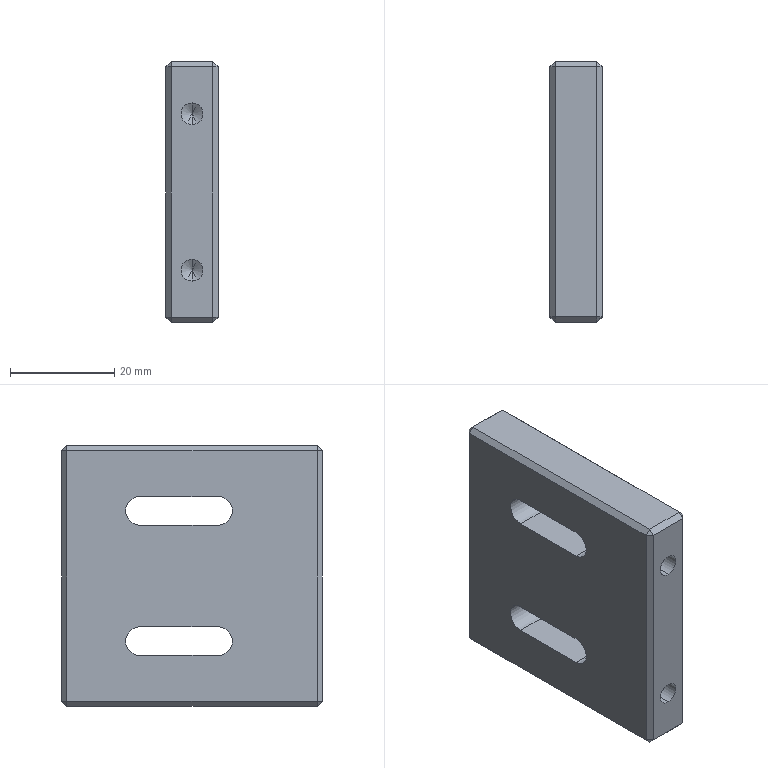Part | STEP file | 01-13 Coil feed support base plate | 1 solid | 42 faces | box 10 x 50 x 50 mm | volume 22250 mm3 | plane 30 | cylinder 8 | cone 4 | commonest cylinder face diameters 4.2 x4 5.5 x4